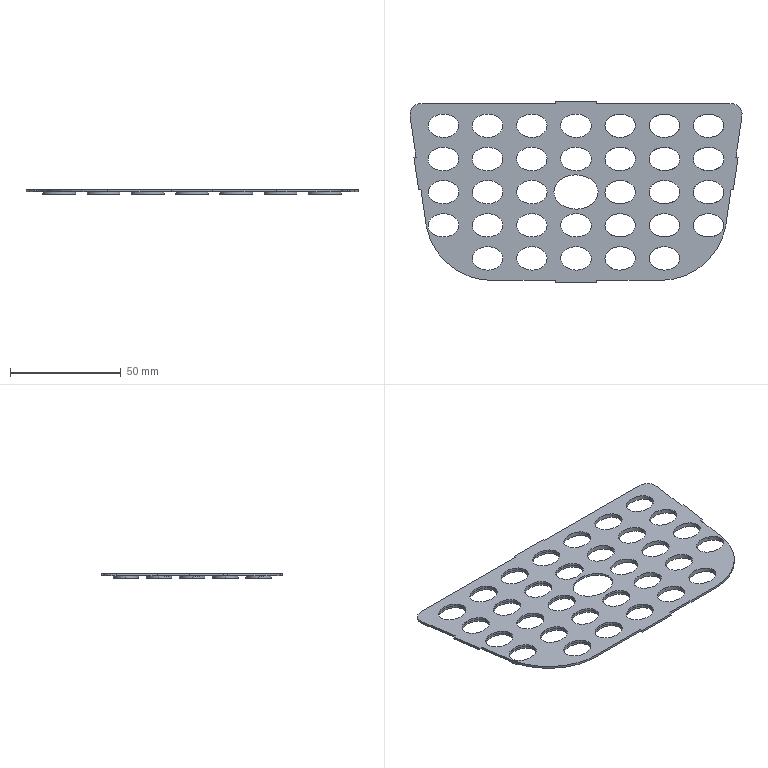Part | SolidWorks | features SplitBody 1 | 1 solid | 226 faces | box 150.242 x 82 x 2 mm | volume 7695 mm3 | spline 168 | plane 56 | cylinder 2 | commonest cylinder face diameters 10 x2